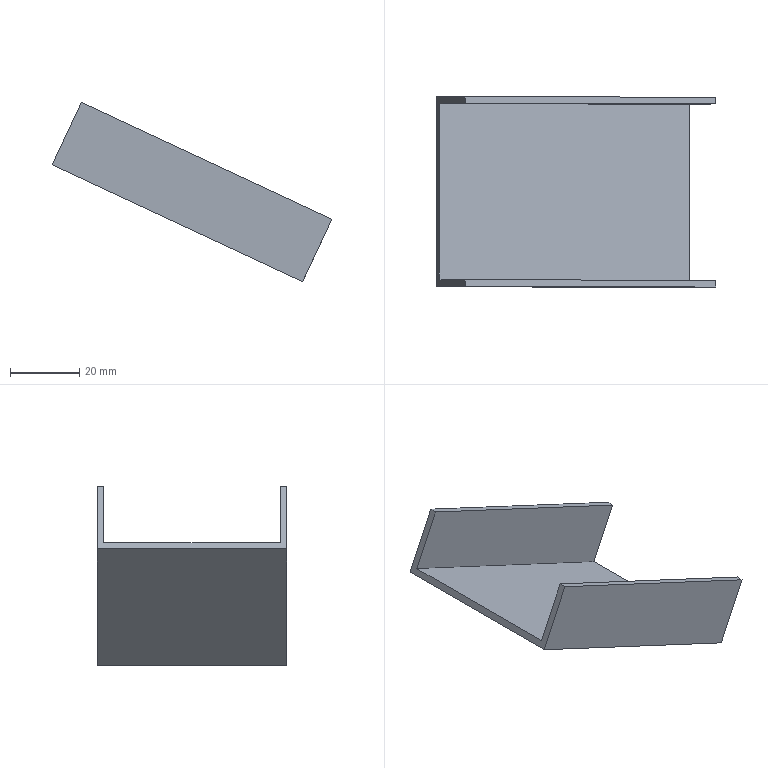Part | NX | features solid 2 | 1 solid | 10 faces | box 80.957 x 55 x 51.936 mm | volume 14560 mm3 | plane 10
STEP:
#1=CARTESIAN_POINT('',(580.,-38.,-290.));
#2=VERTEX_POINT('',#1);
#3=CARTESIAN_POINT('',(580.,13.,-290.));
#4=VERTEX_POINT('',#3);
#5=CARTESIAN_POINT('',(580.,-75.,-290.));
#6=DIRECTION('',(0.,1.,0.));
#7=VECTOR('',#6,1000.);
#8=LINE('',#5,#7);
#9=EDGE_CURVE('',#2,#4,#8,.T.);
#10=ORIENTED_EDGE('',*,*,#9,.F.);
#11=CARTESIAN_POINT('',(652.505,-38.,-323.809));
#12=VERTEX_POINT('',#11);
#13=CARTESIAN_POINT('',(580.,-38.,-290.));
#14=DIRECTION('',(0.9063,0.,-0.4226));
#15=VECTOR('',#14,1000.);
#16=LINE('',#13,#15);
#17=EDGE_CURVE('',#2,#12,#16,.T.);
#18=ORIENTED_EDGE('',*,*,#17,.T.);
#19=CARTESIAN_POINT('',(652.505,13.,-323.809));
#20=VERTEX_POINT('',#19);
#21=CARTESIAN_POINT('',(652.505,-75.,-323.809));
#22=DIRECTION('',(0.,-1.,0.));
#23=VECTOR('',#22,1000.);
#24=LINE('',#21,#23);
#25=EDGE_CURVE('',#12,#20,#24,.F.);
#26=ORIENTED_EDGE('',*,*,#25,.T.);
#27=CARTESIAN_POINT('',(580.,13.,-290.));
#28=DIRECTION('',(0.9063,0.,-0.4226));
#29=VECTOR('',#28,1000.);
#30=LINE('',#27,#29);
#31=EDGE_CURVE('',#4,#20,#30,.T.);
#32=ORIENTED_EDGE('',*,*,#31,.F.);
#33=EDGE_LOOP('',(#10,#18,#26,#32));
#34=FACE_BOUND('',#33,.T.);
#35=CARTESIAN_POINT('',(580.,-75.,-290.));
#36=DIRECTION('',(-0.4226,0.,-0.9063));
#37=DIRECTION('',(-0.9063,0.,0.4226));
#38=AXIS2_PLACEMENT_3D('',#35,#36,#37);
#39=PLANE('',#38);
#40=ADVANCED_FACE('',(#34),#39,.F.);
#41=CARTESIAN_POINT('',(587.607,15.,-273.686));
#42=VERTEX_POINT('',#41);
#43=CARTESIAN_POINT('',(579.155,15.,-291.813));
#44=VERTEX_POINT('',#43);
#45=CARTESIAN_POINT('',(580.,15.,-290.));
#46=DIRECTION('',(-0.4226,0.,-0.9063));
#47=VECTOR('',#46,1000.);
#48=LINE('',#45,#47);
#49=EDGE_CURVE('',#42,#44,#48,.T.);
#50=ORIENTED_EDGE('',*,*,#49,.T.);
#51=CARTESIAN_POINT('',(579.155,-40.,-291.813));
#52=VERTEX_POINT('',#51);
#53=CARTESIAN_POINT('',(579.155,-75.,-291.813));
#54=DIRECTION('',(0.,1.,0.));
#55=VECTOR('',#54,1000.);
#56=LINE('',#53,#55);
#57=EDGE_CURVE('',#52,#44,#56,.T.);
#58=ORIENTED_EDGE('',*,*,#57,.F.);
#59=CARTESIAN_POINT('',(587.607,-40.,-273.686));
#60=VERTEX_POINT('',#59);
#61=CARTESIAN_POINT('',(603.566,-40.,-239.463));
#62=DIRECTION('',(-0.4226,0.,-0.9063));
#63=VECTOR('',#62,1000.);
#64=LINE('',#61,#63);
#65=EDGE_CURVE('',#60,#52,#64,.T.);
#66=ORIENTED_EDGE('',*,*,#65,.F.);
#67=CARTESIAN_POINT('',(587.607,-38.,-273.686));
#68=VERTEX_POINT('',#67);
#69=CARTESIAN_POINT('',(587.607,-45.,-273.686));
#70=DIRECTION('',(0.,-1.,0.));
#71=VECTOR('',#70,1000.);
#72=LINE('',#69,#71);
#73=EDGE_CURVE('',#60,#68,#72,.F.);
#74=ORIENTED_EDGE('',*,*,#73,.T.);
#75=CARTESIAN_POINT('',(580.,-38.,-290.));
#76=DIRECTION('',(-0.4226,0.,-0.9063));
#77=VECTOR('',#76,1000.);
#78=LINE('',#75,#77);
#79=EDGE_CURVE('',#68,#2,#78,.T.);
#80=ORIENTED_EDGE('',*,*,#79,.T.);
#81=ORIENTED_EDGE('',*,*,#9,.T.);
#82=CARTESIAN_POINT('',(587.607,13.,-273.686));
#83=VERTEX_POINT('',#82);
#84=CARTESIAN_POINT('',(587.607,13.,-273.686));
#85=DIRECTION('',(-0.4226,0.,-0.9063));
#86=VECTOR('',#85,1000.);
#87=LINE('',#84,#86);
#88=EDGE_CURVE('',#83,#4,#87,.T.);
#89=ORIENTED_EDGE('',*,*,#88,.F.);
#90=CARTESIAN_POINT('',(587.607,13.,-273.686));
#91=DIRECTION('',(0.,-1.,0.));
#92=VECTOR('',#91,1000.);
#93=LINE('',#90,#92);
#94=EDGE_CURVE('',#83,#42,#93,.F.);
#95=ORIENTED_EDGE('',*,*,#94,.T.);
#96=EDGE_LOOP('',(#50,#58,#66,#74,#80,#81,#89,#95));
#97=FACE_BOUND('',#96,.T.);
#98=CARTESIAN_POINT('',(580.,-75.,-290.));
#99=DIRECTION('',(-0.9063,0.,0.4226));
#100=DIRECTION('',(0.,1.,0.));
#101=AXIS2_PLACEMENT_3D('',#98,#99,#100);
#102=PLANE('',#101);
#103=ADVANCED_FACE('',(#97),#102,.T.);
#104=ORIENTED_EDGE('',*,*,#49,.F.);
#105=CARTESIAN_POINT('',(660.112,15.,-307.496));
#106=VERTEX_POINT('',#105);
#107=CARTESIAN_POINT('',(587.607,15.,-273.686));
#108=DIRECTION('',(0.9063,0.,-0.4226));
#109=VECTOR('',#108,1000.);
#110=LINE('',#107,#109);
#111=EDGE_CURVE('',#42,#106,#110,.T.);
#112=ORIENTED_EDGE('',*,*,#111,.T.);
#113=CARTESIAN_POINT('',(651.659,15.,-325.622));
#114=VERTEX_POINT('',#113);
#115=CARTESIAN_POINT('',(652.505,15.,-323.809));
#116=DIRECTION('',(0.4226,0.,0.9063));
#117=VECTOR('',#116,1000.);
#118=LINE('',#115,#117);
#119=EDGE_CURVE('',#106,#114,#118,.F.);
#120=ORIENTED_EDGE('',*,*,#119,.T.);
#121=CARTESIAN_POINT('',(579.155,15.,-291.813));
#122=DIRECTION('',(0.9063,0.,-0.4226));
#123=VECTOR('',#122,1000.);
#124=LINE('',#121,#123);
#125=EDGE_CURVE('',#44,#114,#124,.T.);
#126=ORIENTED_EDGE('',*,*,#125,.F.);
#127=EDGE_LOOP('',(#104,#112,#120,#126));
#128=FACE_BOUND('',#127,.T.);
#129=CARTESIAN_POINT('',(580.,15.,-290.));
#130=DIRECTION('',(0.,1.,0.));
#131=DIRECTION('',(0.9063,0.,-0.4226));
#132=AXIS2_PLACEMENT_3D('',#129,#130,#131);
#133=PLANE('',#132);
#134=ADVANCED_FACE('',(#128),#133,.T.);
#135=ORIENTED_EDGE('',*,*,#25,.F.);
#136=CARTESIAN_POINT('',(660.112,-38.,-307.496));
#137=VERTEX_POINT('',#136);
#138=CARTESIAN_POINT('',(660.112,-38.,-307.496));
#139=DIRECTION('',(0.4226,0.,0.9063));
#140=VECTOR('',#139,1000.);
#141=LINE('',#138,#140);
#142=EDGE_CURVE('',#137,#12,#141,.F.);
#143=ORIENTED_EDGE('',*,*,#142,.F.);
#144=CARTESIAN_POINT('',(660.112,-40.,-307.496));
#145=VERTEX_POINT('',#144);
#146=CARTESIAN_POINT('',(660.112,-45.,-307.496));
#147=DIRECTION('',(0.,-1.,0.));
#148=VECTOR('',#147,1000.);
#149=LINE('',#146,#148);
#150=EDGE_CURVE('',#145,#137,#149,.F.);
#151=ORIENTED_EDGE('',*,*,#150,.F.);
#152=CARTESIAN_POINT('',(651.659,-40.,-325.622));
#153=VERTEX_POINT('',#152);
#154=CARTESIAN_POINT('',(652.505,-40.,-323.809));
#155=DIRECTION('',(0.4226,0.,0.9063));
#156=VECTOR('',#155,1000.);
#157=LINE('',#154,#156);
#158=EDGE_CURVE('',#145,#153,#157,.F.);
#159=ORIENTED_EDGE('',*,*,#158,.T.);
#160=CARTESIAN_POINT('',(651.659,-75.,-325.622));
#161=DIRECTION('',(0.,-1.,0.));
#162=VECTOR('',#161,1000.);
#163=LINE('',#160,#162);
#164=EDGE_CURVE('',#153,#114,#163,.F.);
#165=ORIENTED_EDGE('',*,*,#164,.T.);
#166=ORIENTED_EDGE('',*,*,#119,.F.);
#167=CARTESIAN_POINT('',(660.112,13.,-307.496));
#168=VERTEX_POINT('',#167);
#169=CARTESIAN_POINT('',(660.112,13.,-307.496));
#170=DIRECTION('',(0.,-1.,0.));
#171=VECTOR('',#170,1000.);
#172=LINE('',#169,#171);
#173=EDGE_CURVE('',#168,#106,#172,.F.);
#174=ORIENTED_EDGE('',*,*,#173,.F.);
#175=CARTESIAN_POINT('',(660.112,13.,-307.496));
#176=DIRECTION('',(-0.4226,0.,-0.9063));
#177=VECTOR('',#176,1000.);
#178=LINE('',#175,#177);
#179=EDGE_CURVE('',#168,#20,#178,.T.);
#180=ORIENTED_EDGE('',*,*,#179,.T.);
#181=EDGE_LOOP('',(#135,#143,#151,#159,#165,#166,#174,#180));
#182=FACE_BOUND('',#181,.T.);
#183=CARTESIAN_POINT('',(652.505,-75.,-323.809));
#184=DIRECTION('',(-0.9063,0.,0.4226));
#185=DIRECTION('',(0.,1.,0.));
#186=AXIS2_PLACEMENT_3D('',#183,#184,#185);
#187=PLANE('',#186);
#188=ADVANCED_FACE('',(#182),#187,.F.);
#189=ORIENTED_EDGE('',*,*,#125,.T.);
#190=ORIENTED_EDGE('',*,*,#164,.F.);
#191=CARTESIAN_POINT('',(762.589,-40.,-377.349));
#192=DIRECTION('',(0.9063,0.,-0.4226));
#193=VECTOR('',#192,1000.);
#194=LINE('',#191,#193);
#195=EDGE_CURVE('',#52,#153,#194,.T.);
#196=ORIENTED_EDGE('',*,*,#195,.F.);
#197=ORIENTED_EDGE('',*,*,#57,.T.);
#198=EDGE_LOOP('',(#189,#190,#196,#197));
#199=FACE_BOUND('',#198,.T.);
#200=CARTESIAN_POINT('',(579.155,-75.,-291.813));
#201=DIRECTION('',(-0.4226,0.,-0.9063));
#202=DIRECTION('',(-0.9063,0.,0.4226));
#203=AXIS2_PLACEMENT_3D('',#200,#201,#202);
#204=PLANE('',#203);
#205=ADVANCED_FACE('',(#199),#204,.T.);
#206=ORIENTED_EDGE('',*,*,#158,.F.);
#207=CARTESIAN_POINT('',(771.041,-40.,-359.223));
#208=DIRECTION('',(-0.9063,0.,0.4226));
#209=VECTOR('',#208,1000.);
#210=LINE('',#207,#209);
#211=EDGE_CURVE('',#60,#145,#210,.F.);
#212=ORIENTED_EDGE('',*,*,#211,.F.);
#213=ORIENTED_EDGE('',*,*,#65,.T.);
#214=ORIENTED_EDGE('',*,*,#195,.T.);
#215=EDGE_LOOP('',(#206,#212,#213,#214));
#216=FACE_BOUND('',#215,.T.);
#217=CARTESIAN_POINT('',(787.,-40.,-325.));
#218=DIRECTION('',(0.,-1.,0.));
#219=DIRECTION('',(0.,0.,-1.));
#220=AXIS2_PLACEMENT_3D('',#217,#218,#219);
#221=PLANE('',#220);
#222=ADVANCED_FACE('',(#216),#221,.T.);
#223=ORIENTED_EDGE('',*,*,#88,.T.);
#224=ORIENTED_EDGE('',*,*,#31,.T.);
#225=ORIENTED_EDGE('',*,*,#179,.F.);
#226=CARTESIAN_POINT('',(587.607,13.,-273.686));
#227=DIRECTION('',(0.9063,0.,-0.4226));
#228=VECTOR('',#227,1000.);
#229=LINE('',#226,#228);
#230=EDGE_CURVE('',#83,#168,#229,.T.);
#231=ORIENTED_EDGE('',*,*,#230,.F.);
#232=EDGE_LOOP('',(#223,#224,#225,#231));
#233=FACE_BOUND('',#232,.T.);
#234=CARTESIAN_POINT('',(587.607,13.,-273.686));
#235=DIRECTION('',(0.,1.,0.));
#236=DIRECTION('',(0.,0.,1.));
#237=AXIS2_PLACEMENT_3D('',#234,#235,#236);
#238=PLANE('',#237);
#239=ADVANCED_FACE('',(#233),#238,.F.);
#240=ORIENTED_EDGE('',*,*,#173,.T.);
#241=ORIENTED_EDGE('',*,*,#111,.F.);
#242=ORIENTED_EDGE('',*,*,#94,.F.);
#243=ORIENTED_EDGE('',*,*,#230,.T.);
#244=EDGE_LOOP('',(#240,#241,#242,#243));
#245=FACE_BOUND('',#244,.T.);
#246=CARTESIAN_POINT('',(587.607,13.,-273.686));
#247=DIRECTION('',(0.4226,0.,0.9063));
#248=DIRECTION('',(0.9063,0.,-0.4226));
#249=AXIS2_PLACEMENT_3D('',#246,#247,#248);
#250=PLANE('',#249);
#251=ADVANCED_FACE('',(#245),#250,.T.);
#252=ORIENTED_EDGE('',*,*,#17,.F.);
#253=ORIENTED_EDGE('',*,*,#79,.F.);
#254=CARTESIAN_POINT('',(587.607,-38.,-273.686));
#255=DIRECTION('',(-0.9063,0.,0.4226));
#256=VECTOR('',#255,1000.);
#257=LINE('',#254,#256);
#258=EDGE_CURVE('',#68,#137,#257,.F.);
#259=ORIENTED_EDGE('',*,*,#258,.T.);
#260=ORIENTED_EDGE('',*,*,#142,.T.);
#261=EDGE_LOOP('',(#252,#253,#259,#260));
#262=FACE_BOUND('',#261,.T.);
#263=CARTESIAN_POINT('',(587.607,-38.,-273.686));
#264=DIRECTION('',(0.,1.,0.));
#265=DIRECTION('',(0.,0.,1.));
#266=AXIS2_PLACEMENT_3D('',#263,#264,#265);
#267=PLANE('',#266);
#268=ADVANCED_FACE('',(#262),#267,.T.);
#269=ORIENTED_EDGE('',*,*,#150,.T.);
#270=ORIENTED_EDGE('',*,*,#258,.F.);
#271=ORIENTED_EDGE('',*,*,#73,.F.);
#272=ORIENTED_EDGE('',*,*,#211,.T.);
#273=EDGE_LOOP('',(#269,#270,#271,#272));
#274=FACE_BOUND('',#273,.T.);
#275=CARTESIAN_POINT('',(587.607,-45.,-273.686));
#276=DIRECTION('',(0.4226,0.,0.9063));
#277=DIRECTION('',(0.9063,0.,-0.4226));
#278=AXIS2_PLACEMENT_3D('',#275,#276,#277);
#279=PLANE('',#278);
#280=ADVANCED_FACE('',(#274),#279,.T.);
#281=CLOSED_SHELL('',(#40,#103,#134,#188,#205,#222,#239,#251,#268,#280));
#282=MANIFOLD_SOLID_BREP('',#281);
#283=(LENGTH_UNIT()NAMED_UNIT(*)SI_UNIT(.MILLI.,.METRE.));
#284=UNCERTAINTY_MEASURE_WITH_UNIT(LENGTH_MEASURE(0.00001),#283,'','');
#285=(NAMED_UNIT(*)PLANE_ANGLE_UNIT()SI_UNIT($,.RADIAN.));
#286=(NAMED_UNIT(*)SI_UNIT($,.STERADIAN.)SOLID_ANGLE_UNIT());
#287=(GEOMETRIC_REPRESENTATION_CONTEXT(3)GLOBAL_UNCERTAINTY_ASSIGNED_CONTEXT((#284))GLOBAL_UNIT_ASSIGNED_CONTEXT((#283,#285,#286))REPRESENTATION_CONTEXT('',''));
#288=ADVANCED_BREP_SHAPE_REPRESENTATION('',(#282),#287);